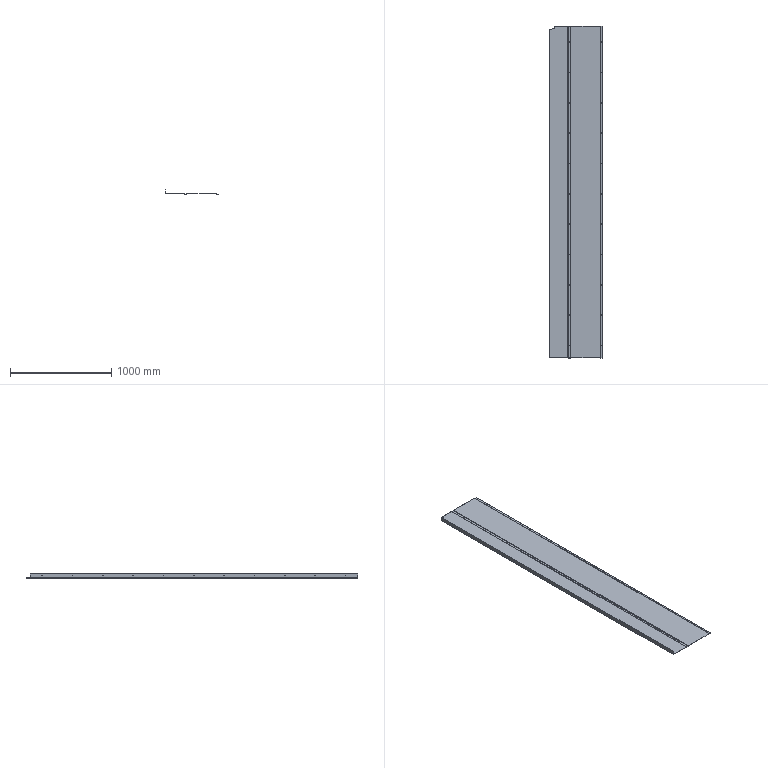Part | STEP file | TS-S85 | 1 solid | 135 faces | box 528 x 3283 x 43 mm | volume 2240757 mm3 | cylinder 83 | plane 52 | commonest cylinder face diameters 5.4 x66 0.4 x7 2.8 x7 10 x1 16 x1 18 x1